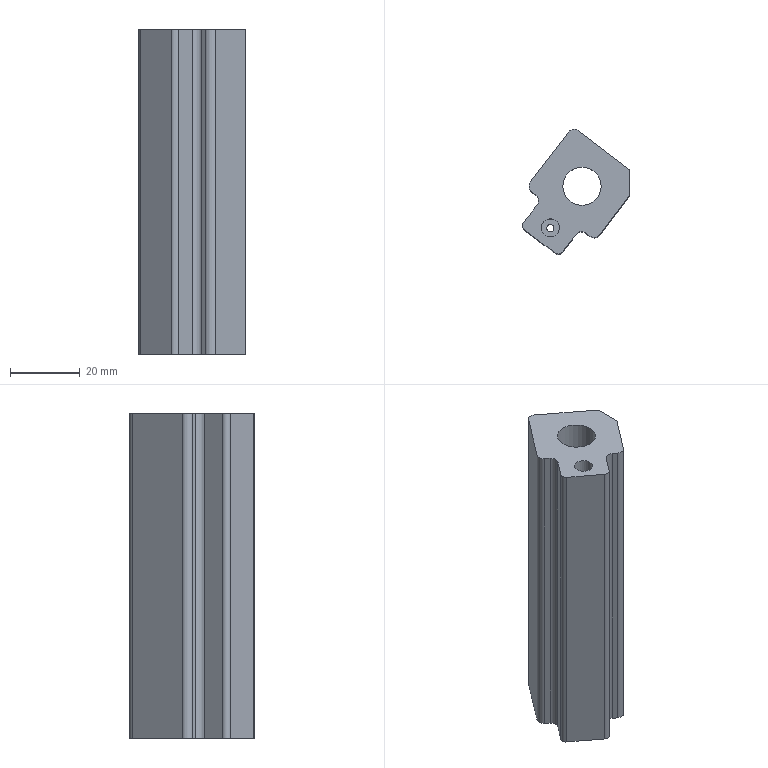Part | STEP file | gslz 2016.10.28-10_id2874_x_t | 1 solid | 24 faces | box 30.689 x 35.785 x 93 mm | volume 42819 mm3 | plane 12 | cylinder 11 | spline 1 | commonest cylinder face diameters 4 x5 3 x2 2.1 x1 5.2 x1 11 x1 17 x1